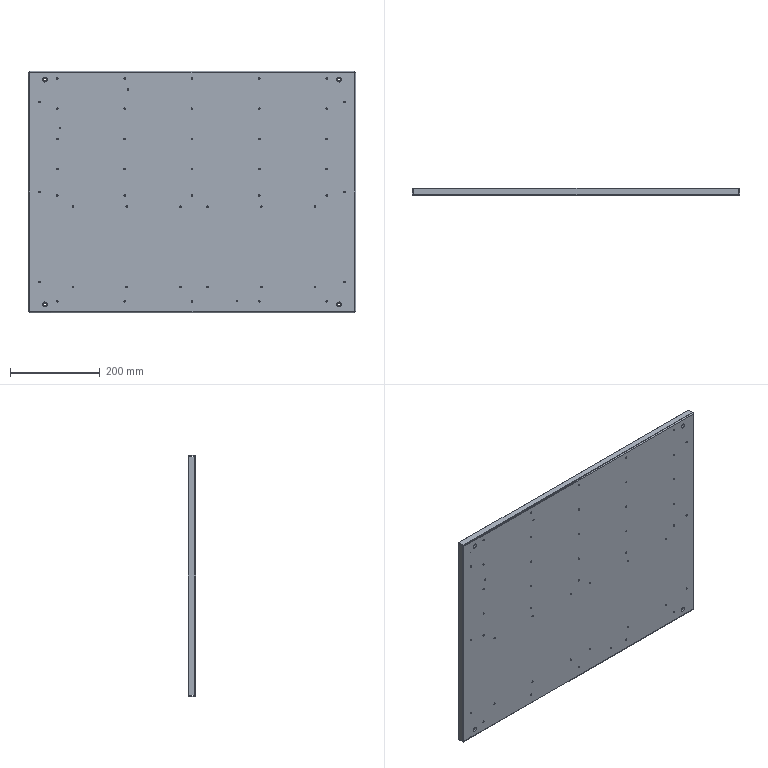Part | SolidWorks | features HoleWzd 7, ICE 2, LPattern 2, EdgeFlange 1, FlatPattern 1, SMBaseFlange 1, SheetMetal 1 | 1 solid | 180 faces | box 729 x 16 x 537 mm | volume 887754 mm3 | cylinder 126 | plane 46 | spline 8 | commonest cylinder face diameters 3.3 x100 6 x8 10 x8 1.473 x4 5.473 x4 2.5 x2